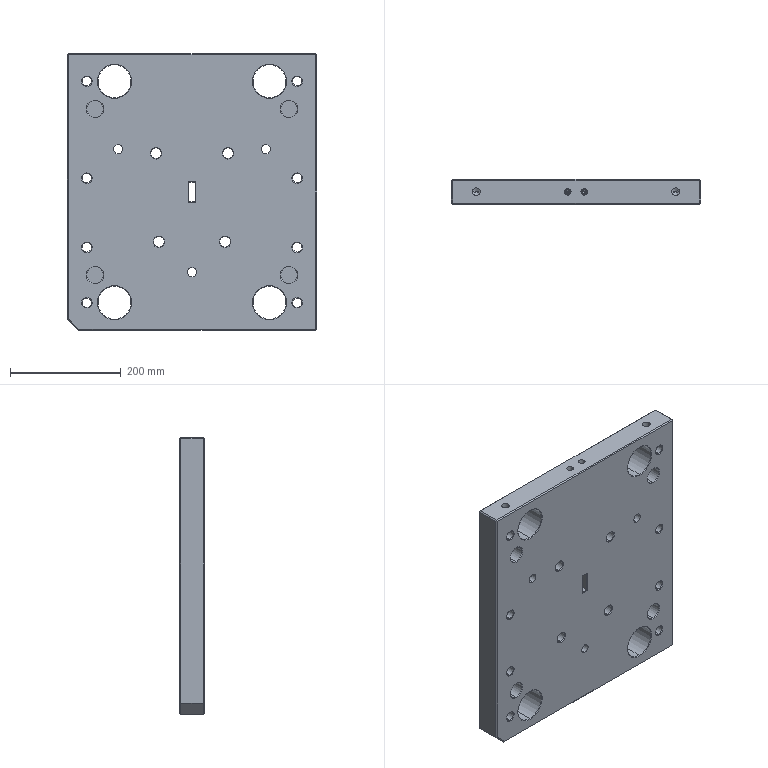Part | STEP file | PS - 1 cav | 1 solid | 209 faces | box 450 x 45 x 500 mm | volume 9255864 mm3 | cone 94 | cylinder 68 | plane 47 | commonest cylinder face diameters 17 x16 14 x8 19 x8 30 x8 60 x8 16.5 x6